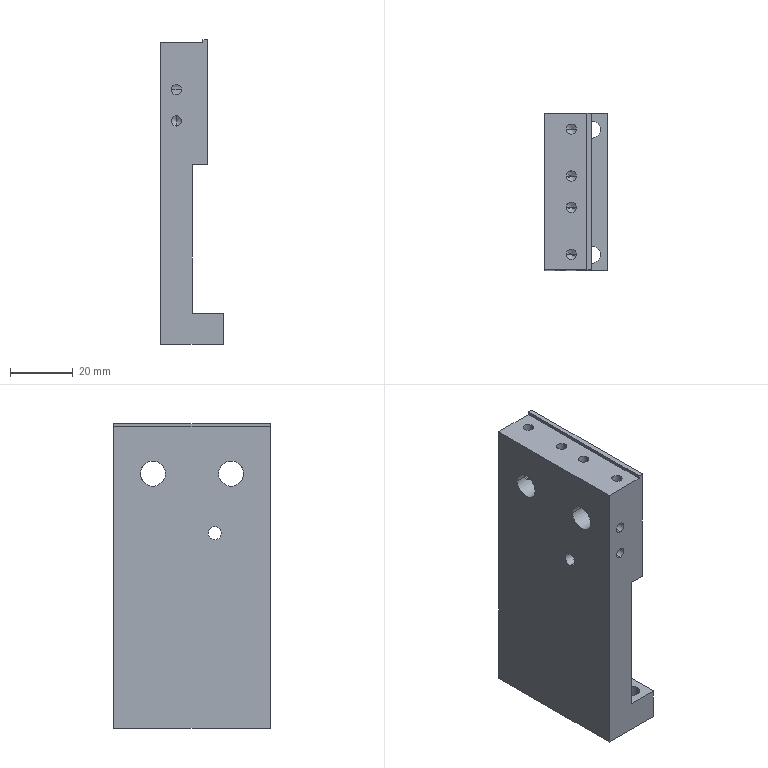Part | STEP file | 11-FG-B00811 | 1 solid | 50 faces | box 20 x 50 x 97.4 mm | volume 60152 mm3 | cylinder 26 | cone 12 | plane 12 | commonest cylinder face diameters 3.3 x16 5.5 x4 8 x4 4.2 x2